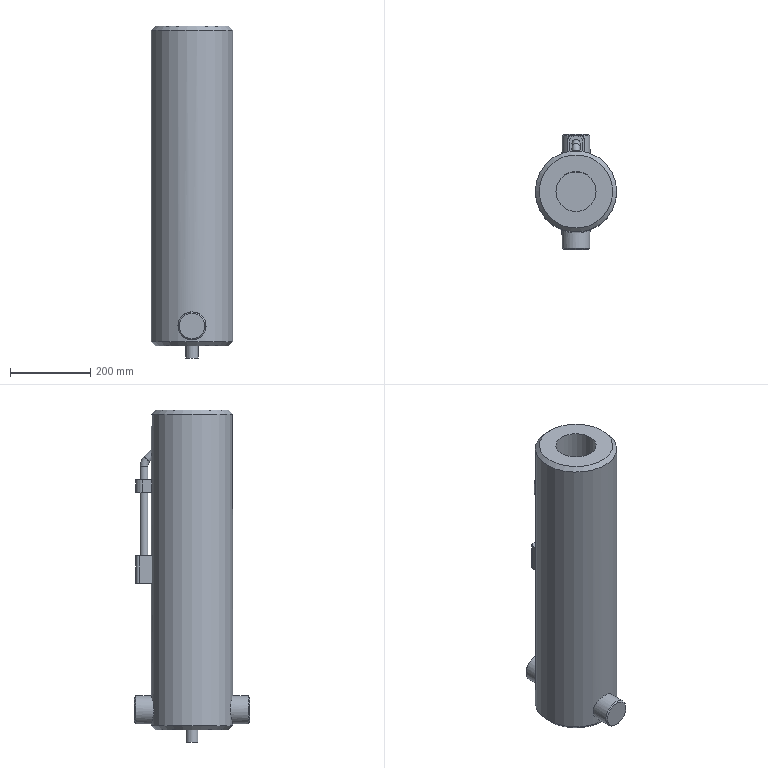Part | NX | features 护帮千斤顶缸 2 | 1 solid | 38 faces | box 203 x 287 x 828 mm | volume 20904449 mm3 | plane 17 | cylinder 14 | cone 6 | torus 1 | commonest cylinder face diameters 20 x3 10 x2 16 x2 34 x2 70 x2 30 x1
STEP:
#1=CARTESIAN_POINT('',(91.5,0.,0.));
#2=VERTEX_POINT('',#1);
#3=CARTESIAN_POINT('',(0.,0.,0.));
#4=DIRECTION('',(0.,0.,1.));
#5=DIRECTION('',(1.,0.,0.));
#6=AXIS2_PLACEMENT_3D('',#3,#4,#5);
#7=CIRCLE('',#6,91.5);
#8=EDGE_CURVE('',#2,#2,#7,.F.);
#9=ORIENTED_EDGE('',*,*,#8,.T.);
#10=EDGE_LOOP('',(#9));
#11=FACE_BOUND('',#10,.T.);
#12=CARTESIAN_POINT('',(15.,0.,0.));
#13=VERTEX_POINT('',#12);
#14=CARTESIAN_POINT('',(0.,0.,0.));
#15=DIRECTION('',(0.,0.,1.));
#16=DIRECTION('',(1.,0.,0.));
#17=AXIS2_PLACEMENT_3D('',#14,#15,#16);
#18=CIRCLE('',#17,15.);
#19=EDGE_CURVE('',#13,#13,#18,.F.);
#20=ORIENTED_EDGE('',*,*,#19,.F.);
#21=EDGE_LOOP('',(#20));
#22=FACE_BOUND('',#21,.T.);
#23=CARTESIAN_POINT('',(0.,0.,0.));
#24=DIRECTION('',(0.,0.,1.));
#25=DIRECTION('',(1.,0.,0.));
#26=AXIS2_PLACEMENT_3D('',#23,#24,#25);
#27=PLANE('',#26);
#28=ADVANCED_FACE('',(#11,#22),#27,.F.);
#29=CARTESIAN_POINT('',(20.,132.,434.5));
#30=VERTEX_POINT('',#29);
#31=CARTESIAN_POINT('',(20.,99.51,434.5));
#32=VERTEX_POINT('',#31);
#33=CARTESIAN_POINT('',(20.,140.,434.5));
#34=DIRECTION('',(0.,-1.,0.));
#35=VECTOR('',#34,1000.);
#36=LINE('',#33,#35);
#37=EDGE_CURVE('',#30,#32,#36,.T.);
#38=ORIENTED_EDGE('',*,*,#37,.F.);
#39=CARTESIAN_POINT('',(12.,140.,434.5));
#40=VERTEX_POINT('',#39);
#41=CARTESIAN_POINT('',(12.,132.,434.5));
#42=DIRECTION('',(0.,0.,-1.));
#43=DIRECTION('',(-1.,0.,0.));
#44=AXIS2_PLACEMENT_3D('',#41,#42,#43);
#45=CIRCLE('',#44,8.);
#46=EDGE_CURVE('',#30,#40,#45,.F.);
#47=ORIENTED_EDGE('',*,*,#46,.T.);
#48=CARTESIAN_POINT('',(-12.,140.,434.5));
#49=VERTEX_POINT('',#48);
#50=CARTESIAN_POINT('',(-20.,140.,434.5));
#51=DIRECTION('',(1.,0.,0.));
#52=VECTOR('',#51,1000.);
#53=LINE('',#50,#52);
#54=EDGE_CURVE('',#49,#40,#53,.T.);
#55=ORIENTED_EDGE('',*,*,#54,.F.);
#56=CARTESIAN_POINT('',(-20.,132.,434.5));
#57=VERTEX_POINT('',#56);
#58=CARTESIAN_POINT('',(-12.,132.,434.5));
#59=DIRECTION('',(0.,0.,-1.));
#60=DIRECTION('',(-1.,0.,0.));
#61=AXIS2_PLACEMENT_3D('',#58,#59,#60);
#62=CIRCLE('',#61,8.);
#63=EDGE_CURVE('',#49,#57,#62,.F.);
#64=ORIENTED_EDGE('',*,*,#63,.T.);
#65=CARTESIAN_POINT('',(-20.,99.51,434.5));
#66=VERTEX_POINT('',#65);
#67=CARTESIAN_POINT('',(-20.,140.,434.5));
#68=DIRECTION('',(0.,-1.,0.));
#69=VECTOR('',#68,1000.);
#70=LINE('',#67,#69);
#71=EDGE_CURVE('',#57,#66,#70,.T.);
#72=ORIENTED_EDGE('',*,*,#71,.T.);
#73=CARTESIAN_POINT('',(0.,0.,434.5));
#74=DIRECTION('',(0.,0.,-1.));
#75=DIRECTION('',(-1.,0.,0.));
#76=AXIS2_PLACEMENT_3D('',#73,#74,#75);
#77=CIRCLE('',#76,101.5);
#78=EDGE_CURVE('',#66,#32,#77,.T.);
#79=ORIENTED_EDGE('',*,*,#78,.T.);
#80=EDGE_LOOP('',(#38,#47,#55,#64,#72,#79));
#81=FACE_BOUND('',#80,.T.);
#82=CARTESIAN_POINT('',(10.,119.755,434.5));
#83=VERTEX_POINT('',#82);
#84=CARTESIAN_POINT('',(0.,119.755,434.5));
#85=DIRECTION('',(0.,0.,1.));
#86=DIRECTION('',(1.,0.,0.));
#87=AXIS2_PLACEMENT_3D('',#84,#85,#86);
#88=CIRCLE('',#87,10.);
#89=EDGE_CURVE('',#83,#83,#88,.T.);
#90=ORIENTED_EDGE('',*,*,#89,.F.);
#91=EDGE_LOOP('',(#90));
#92=FACE_BOUND('',#91,.T.);
#93=CARTESIAN_POINT('',(-20.,140.,434.5));
#94=DIRECTION('',(0.,0.,-1.));
#95=DIRECTION('',(-1.,0.,0.));
#96=AXIS2_PLACEMENT_3D('',#93,#94,#95);
#97=PLANE('',#96);
#98=ADVANCED_FACE('',(#81,#92),#97,.F.);
#99=CARTESIAN_POINT('',(17.,123.,624.17));
#100=VERTEX_POINT('',#99);
#101=CARTESIAN_POINT('',(17.,100.066,624.17));
#102=VERTEX_POINT('',#101);
#103=CARTESIAN_POINT('',(17.,140.,624.17));
#104=DIRECTION('',(0.,-1.,0.));
#105=VECTOR('',#104,1000.);
#106=LINE('',#103,#105);
#107=EDGE_CURVE('',#100,#102,#106,.T.);
#108=ORIENTED_EDGE('',*,*,#107,.F.);
#109=CARTESIAN_POINT('',(0.,140.,624.17));
#110=VERTEX_POINT('',#109);
#111=CARTESIAN_POINT('',(0.,123.,624.17));
#112=DIRECTION('',(0.,0.,-1.));
#113=DIRECTION('',(-1.,0.,0.));
#114=AXIS2_PLACEMENT_3D('',#111,#112,#113);
#115=CIRCLE('',#114,17.);
#116=EDGE_CURVE('',#100,#110,#115,.F.);
#117=ORIENTED_EDGE('',*,*,#116,.T.);
#118=CARTESIAN_POINT('',(-17.,123.,624.17));
#119=VERTEX_POINT('',#118);
#120=CARTESIAN_POINT('',(0.,123.,624.17));
#121=DIRECTION('',(0.,0.,-1.));
#122=DIRECTION('',(-1.,0.,0.));
#123=AXIS2_PLACEMENT_3D('',#120,#121,#122);
#124=CIRCLE('',#123,17.);
#125=EDGE_CURVE('',#110,#119,#124,.F.);
#126=ORIENTED_EDGE('',*,*,#125,.T.);
#127=CARTESIAN_POINT('',(-17.,100.066,624.17));
#128=VERTEX_POINT('',#127);
#129=CARTESIAN_POINT('',(-17.,140.,624.17));
#130=DIRECTION('',(0.,-1.,0.));
#131=VECTOR('',#130,1000.);
#132=LINE('',#129,#131);
#133=EDGE_CURVE('',#119,#128,#132,.T.);
#134=ORIENTED_EDGE('',*,*,#133,.T.);
#135=CARTESIAN_POINT('',(0.,0.,624.17));
#136=DIRECTION('',(0.,0.,-1.));
#137=DIRECTION('',(-1.,0.,0.));
#138=AXIS2_PLACEMENT_3D('',#135,#136,#137);
#139=CIRCLE('',#138,101.5);
#140=EDGE_CURVE('',#128,#102,#139,.T.);
#141=ORIENTED_EDGE('',*,*,#140,.T.);
#142=EDGE_LOOP('',(#108,#117,#126,#134,#141));
#143=FACE_BOUND('',#142,.T.);
#144=CARTESIAN_POINT('',(-10.,119.755,624.17));
#145=VERTEX_POINT('',#144);
#146=CARTESIAN_POINT('',(0.,119.755,624.17));
#147=DIRECTION('',(0.,0.,-1.));
#148=DIRECTION('',(-1.,0.,0.));
#149=AXIS2_PLACEMENT_3D('',#146,#147,#148);
#150=CIRCLE('',#149,10.);
#151=EDGE_CURVE('',#145,#145,#150,.F.);
#152=ORIENTED_EDGE('',*,*,#151,.F.);
#153=EDGE_LOOP('',(#152));
#154=FACE_BOUND('',#153,.T.);
#155=CARTESIAN_POINT('',(-17.,140.,624.17));
#156=DIRECTION('',(0.,0.,-1.));
#157=DIRECTION('',(-1.,0.,0.));
#158=AXIS2_PLACEMENT_3D('',#155,#156,#157);
#159=PLANE('',#158);
#160=ADVANCED_FACE('',(#143,#154),#159,.F.);
#161=CARTESIAN_POINT('',(-17.,123.,591.84));
#162=VERTEX_POINT('',#161);
#163=CARTESIAN_POINT('',(0.,140.,591.84));
#164=VERTEX_POINT('',#163);
#165=CARTESIAN_POINT('',(0.,123.,591.84));
#166=DIRECTION('',(0.,0.,1.));
#167=DIRECTION('',(1.,0.,0.));
#168=AXIS2_PLACEMENT_3D('',#165,#166,#167);
#169=CIRCLE('',#168,17.);
#170=EDGE_CURVE('',#162,#164,#169,.F.);
#171=ORIENTED_EDGE('',*,*,#170,.T.);
#172=CARTESIAN_POINT('',(17.,123.,591.84));
#173=VERTEX_POINT('',#172);
#174=CARTESIAN_POINT('',(0.,123.,591.84));
#175=DIRECTION('',(0.,0.,1.));
#176=DIRECTION('',(1.,0.,0.));
#177=AXIS2_PLACEMENT_3D('',#174,#175,#176);
#178=CIRCLE('',#177,17.);
#179=EDGE_CURVE('',#164,#173,#178,.F.);
#180=ORIENTED_EDGE('',*,*,#179,.T.);
#181=CARTESIAN_POINT('',(17.,100.066,591.84));
#182=VERTEX_POINT('',#181);
#183=CARTESIAN_POINT('',(17.,140.,591.84));
#184=DIRECTION('',(0.,-1.,0.));
#185=VECTOR('',#184,1000.);
#186=LINE('',#183,#185);
#187=EDGE_CURVE('',#173,#182,#186,.T.);
#188=ORIENTED_EDGE('',*,*,#187,.T.);
#189=CARTESIAN_POINT('',(-17.,100.066,591.84));
#190=VERTEX_POINT('',#189);
#191=CARTESIAN_POINT('',(0.,0.,591.84));
#192=DIRECTION('',(0.,0.,1.));
#193=DIRECTION('',(1.,0.,0.));
#194=AXIS2_PLACEMENT_3D('',#191,#192,#193);
#195=CIRCLE('',#194,101.5);
#196=EDGE_CURVE('',#182,#190,#195,.T.);
#197=ORIENTED_EDGE('',*,*,#196,.T.);
#198=CARTESIAN_POINT('',(-17.,140.,591.84));
#199=DIRECTION('',(0.,-1.,0.));
#200=VECTOR('',#199,1000.);
#201=LINE('',#198,#200);
#202=EDGE_CURVE('',#162,#190,#201,.T.);
#203=ORIENTED_EDGE('',*,*,#202,.F.);
#204=EDGE_LOOP('',(#171,#180,#188,#197,#203));
#205=FACE_BOUND('',#204,.T.);
#206=CARTESIAN_POINT('',(10.,119.755,591.84));
#207=VERTEX_POINT('',#206);
#208=CARTESIAN_POINT('',(0.,119.755,591.84));
#209=DIRECTION('',(0.,0.,1.));
#210=DIRECTION('',(1.,0.,0.));
#211=AXIS2_PLACEMENT_3D('',#208,#209,#210);
#212=CIRCLE('',#211,10.);
#213=EDGE_CURVE('',#207,#207,#212,.F.);
#214=ORIENTED_EDGE('',*,*,#213,.F.);
#215=EDGE_LOOP('',(#214));
#216=FACE_BOUND('',#215,.T.);
#217=CARTESIAN_POINT('',(-17.,140.,591.84));
#218=DIRECTION('',(0.,0.,1.));
#219=DIRECTION('',(1.,0.,0.));
#220=AXIS2_PLACEMENT_3D('',#217,#218,#219);
#221=PLANE('',#220);
#222=ADVANCED_FACE('',(#205,#216),#221,.F.);
#223=CARTESIAN_POINT('',(101.5,0.,788.));
#224=VERTEX_POINT('',#223);
#225=CARTESIAN_POINT('',(0.,0.,788.));
#226=DIRECTION('',(0.,0.,1.));
#227=DIRECTION('',(1.,0.,0.));
#228=AXIS2_PLACEMENT_3D('',#225,#226,#227);
#229=CIRCLE('',#228,101.5);
#230=EDGE_CURVE('',#224,#224,#229,.F.);
#231=ORIENTED_EDGE('',*,*,#230,.T.);
#232=EDGE_LOOP('',(#231));
#233=FACE_BOUND('',#232,.T.);
#234=CARTESIAN_POINT('',(0.,101.5,671.943));
#235=VERTEX_POINT('',#234);
#236=CARTESIAN_POINT('',(-2.408,101.48,672.245));
#237=CARTESIAN_POINT('',(0.8153,101.52,671.637));
#238=CARTESIAN_POINT('',(4.704,101.417,673.183));
#239=CARTESIAN_POINT('',(7.766,101.211,676.987));
#240=CARTESIAN_POINT('',(9.529,101.054,681.426));
#241=CARTESIAN_POINT('',(10.182,100.988,686.186));
#242=CARTESIAN_POINT('',(9.719,101.035,690.945));
#243=CARTESIAN_POINT('',(8.008,101.192,695.439));
#244=CARTESIAN_POINT('',(4.799,101.414,699.129));
#245=CARTESIAN_POINT('',(0.04319,101.542,700.764));
#246=CARTESIAN_POINT('',(-4.734,101.417,699.177));
#247=CARTESIAN_POINT('',(-7.971,101.195,695.504));
#248=CARTESIAN_POINT('',(-9.706,101.036,691.009));
#249=CARTESIAN_POINT('',(-10.185,100.987,686.22));
#250=CARTESIAN_POINT('',(-9.534,101.053,681.451));
#251=CARTESIAN_POINT('',(-7.788,101.21,677.014));
#252=CARTESIAN_POINT('',(-5.218,101.381,673.84));
#253=CARTESIAN_POINT('',(-2.408,101.48,672.245));
#254=CARTESIAN_POINT('',(0.8153,101.52,671.637));
#255=CARTESIAN_POINT('',(4.704,101.417,673.183));
#256=B_SPLINE_CURVE_WITH_KNOTS('',3,(#236,#237,#238,#239,#240,#241,#242,#243,#244,#245,#246,#247,#248,#249,#250,#251,#252,#253,#254,#255),.UNSPECIFIED.,.T.,.F.,(1,1,1,1,1,1,1,1,1,1,1,1,1,1,1,1,1,1,1,1,1,1,1,1),(-0.009513,-0.004756,-0.002378,0.,0.004756,0.009513,0.01427,0.01903,0.02378,0.02854,0.03329,0.03805,0.04281,0.04756,0.05232,0.05708,0.06183,0.06659,0.07134,0.07372,0.0761,0.08086,0.08561,0.09037),.UNSPECIFIED.);
#257=EDGE_CURVE('',#235,#235,#256,.T.);
#258=ORIENTED_EDGE('',*,*,#257,.T.);
#259=EDGE_LOOP('',(#258));
#260=FACE_BOUND('',#259,.T.);
#261=CARTESIAN_POINT('',(-20.,99.51,365.5));
#262=VERTEX_POINT('',#261);
#263=CARTESIAN_POINT('',(-20.,99.51,798.));
#264=DIRECTION('',(0.,0.,-1.));
#265=VECTOR('',#264,1000.);
#266=LINE('',#263,#265);
#267=EDGE_CURVE('',#262,#66,#266,.F.);
#268=ORIENTED_EDGE('',*,*,#267,.F.);
#269=CARTESIAN_POINT('',(20.,99.51,365.5));
#270=VERTEX_POINT('',#269);
#271=CARTESIAN_POINT('',(0.,0.,365.5));
#272=DIRECTION('',(0.,0.,1.));
#273=DIRECTION('',(1.,0.,0.));
#274=AXIS2_PLACEMENT_3D('',#271,#272,#273);
#275=CIRCLE('',#274,101.5);
#276=EDGE_CURVE('',#270,#262,#275,.T.);
#277=ORIENTED_EDGE('',*,*,#276,.F.);
#278=CARTESIAN_POINT('',(20.,99.51,798.));
#279=DIRECTION('',(0.,0.,-1.));
#280=VECTOR('',#279,1000.);
#281=LINE('',#278,#280);
#282=EDGE_CURVE('',#32,#270,#281,.T.);
#283=ORIENTED_EDGE('',*,*,#282,.F.);
#284=ORIENTED_EDGE('',*,*,#78,.F.);
#285=EDGE_LOOP('',(#268,#277,#283,#284));
#286=FACE_BOUND('',#285,.T.);
#287=CARTESIAN_POINT('',(101.5,0.,10.));
#288=VERTEX_POINT('',#287);
#289=CARTESIAN_POINT('',(0.,0.,10.));
#290=DIRECTION('',(0.,0.,1.));
#291=DIRECTION('',(1.,0.,0.));
#292=AXIS2_PLACEMENT_3D('',#289,#290,#291);
#293=CIRCLE('',#292,101.5);
#294=EDGE_CURVE('',#288,#288,#293,.T.);
#295=ORIENTED_EDGE('',*,*,#294,.T.);
#296=EDGE_LOOP('',(#295));
#297=FACE_BOUND('',#296,.T.);
#298=CARTESIAN_POINT('',(0.,-101.5,15.));
#299=VERTEX_POINT('',#298);
#300=CARTESIAN_POINT('',(-13.849,-100.835,16.867));
#301=CARTESIAN_POINT('',(-0.001134,-101.833,14.067));
#302=CARTESIAN_POINT('',(13.853,-100.834,16.867));
#303=CARTESIAN_POINT('',(25.391,-98.445,24.635));
#304=CARTESIAN_POINT('',(33.131,-95.991,36.158));
#305=CARTESIAN_POINT('',(35.93,-94.918,49.967));
#306=CARTESIAN_POINT('',(33.147,-95.985,63.826));
#307=CARTESIAN_POINT('',(25.374,-98.45,75.386));
#308=CARTESIAN_POINT('',(13.835,-100.836,83.136));
#309=CARTESIAN_POINT('',(0.01694,-101.831,85.93));
#310=CARTESIAN_POINT('',(-13.822,-100.839,83.145));
#311=CARTESIAN_POINT('',(-25.383,-98.447,75.386));
#312=CARTESIAN_POINT('',(-31.849,-96.4,65.731));
#313=CARTESIAN_POINT('',(-34.534,-95.448,56.956));
#314=CARTESIAN_POINT('',(-35.466,-95.099,47.672));
#315=CARTESIAN_POINT('',(-33.138,-95.987,36.172));
#316=CARTESIAN_POINT('',(-25.383,-98.448,24.623));
#317=CARTESIAN_POINT('',(-13.849,-100.835,16.867));
#318=CARTESIAN_POINT('',(-0.001134,-101.833,14.067));
#319=CARTESIAN_POINT('',(13.853,-100.834,16.867));
#320=B_SPLINE_CURVE_WITH_KNOTS('',3,(#300,#301,#302,#303,#304,#305,#306,#307,#308,#309,#310,#311,#312,#313,#314,#315,#316,#317,#318,#319),.UNSPECIFIED.,.T.,.F.,(1,1,1,1,1,1,1,1,1,1,1,1,1,1,1,1,1,1,1,1,1,1,1,1),(-0.04135,-0.02757,-0.01378,0.,0.01378,0.02757,0.04135,0.05513,0.06892,0.0827,0.09648,0.1103,0.124,0.1378,0.1516,0.1585,0.1654,0.1792,0.193,0.2067,0.2205,0.2343,0.2481,0.2619),.UNSPECIFIED.);
#321=EDGE_CURVE('',#299,#299,#320,.T.);
#322=ORIENTED_EDGE('',*,*,#321,.F.);
#323=EDGE_LOOP('',(#322));
#324=FACE_BOUND('',#323,.T.);
#325=CARTESIAN_POINT('',(0.,101.5,15.));
#326=VERTEX_POINT('',#325);
#327=CARTESIAN_POINT('',(13.849,100.835,16.867));
#328=CARTESIAN_POINT('',(0.001134,101.833,14.067));
#329=CARTESIAN_POINT('',(-13.853,100.834,16.867));
#330=CARTESIAN_POINT('',(-25.391,98.445,24.635));
#331=CARTESIAN_POINT('',(-33.131,95.991,36.158));
#332=CARTESIAN_POINT('',(-35.93,94.918,49.967));
#333=CARTESIAN_POINT('',(-33.147,95.985,63.826));
#334=CARTESIAN_POINT('',(-25.374,98.45,75.386));
#335=CARTESIAN_POINT('',(-13.835,100.836,83.136));
#336=CARTESIAN_POINT('',(-0.01694,101.831,85.93));
#337=CARTESIAN_POINT('',(13.822,100.839,83.145));
#338=CARTESIAN_POINT('',(25.383,98.447,75.386));
#339=CARTESIAN_POINT('',(31.849,96.4,65.731));
#340=CARTESIAN_POINT('',(34.534,95.448,56.956));
#341=CARTESIAN_POINT('',(35.466,95.099,47.672));
#342=CARTESIAN_POINT('',(33.138,95.987,36.172));
#343=CARTESIAN_POINT('',(25.383,98.448,24.623));
#344=CARTESIAN_POINT('',(13.849,100.835,16.867));
#345=CARTESIAN_POINT('',(0.001134,101.833,14.067));
#346=CARTESIAN_POINT('',(-13.853,100.834,16.867));
#347=B_SPLINE_CURVE_WITH_KNOTS('',3,(#327,#328,#329,#330,#331,#332,#333,#334,#335,#336,#337,#338,#339,#340,#341,#342,#343,#344,#345,#346),.UNSPECIFIED.,.T.,.F.,(1,1,1,1,1,1,1,1,1,1,1,1,1,1,1,1,1,1,1,1,1,1,1,1),(-0.04135,-0.02757,-0.01378,0.,0.01378,0.02757,0.04135,0.05513,0.06892,0.0827,0.09648,0.1103,0.124,0.1378,0.1516,0.1585,0.1654,0.1792,0.193,0.2067,0.2205,0.2343,0.2481,0.2619),.UNSPECIFIED.);
#348=EDGE_CURVE('',#326,#326,#347,.T.);
#349=ORIENTED_EDGE('',*,*,#348,.F.);
#350=EDGE_LOOP('',(#349));
#351=FACE_BOUND('',#350,.T.);
#352=CARTESIAN_POINT('',(-17.,100.066,798.));
#353=DIRECTION('',(0.,0.,-1.));
#354=VECTOR('',#353,1000.);
#355=LINE('',#352,#354);
#356=EDGE_CURVE('',#190,#128,#355,.F.);
#357=ORIENTED_EDGE('',*,*,#356,.F.);
#358=ORIENTED_EDGE('',*,*,#196,.F.);
#359=CARTESIAN_POINT('',(17.,100.066,798.));
#360=DIRECTION('',(0.,0.,-1.));
#361=VECTOR('',#360,1000.);
#362=LINE('',#359,#361);
#363=EDGE_CURVE('',#102,#182,#362,.T.);
#364=ORIENTED_EDGE('',*,*,#363,.F.);
#365=ORIENTED_EDGE('',*,*,#140,.F.);
#366=EDGE_LOOP('',(#357,#358,#364,#365));
#367=FACE_BOUND('',#366,.T.);
#368=CARTESIAN_POINT('',(0.,0.,798.));
#369=DIRECTION('',(0.,0.,-1.));
#370=DIRECTION('',(-1.,0.,0.));
#371=AXIS2_PLACEMENT_3D('',#368,#369,#370);
#372=CYLINDRICAL_SURFACE('',#371,101.5);
#373=ADVANCED_FACE('',(#233,#260,#286,#297,#324,#351,#367),#372,.T.);
#374=CARTESIAN_POINT('',(91.5,0.,798.));
#375=VERTEX_POINT('',#374);
#376=CARTESIAN_POINT('',(0.,0.,798.));
#377=DIRECTION('',(0.,0.,1.));
#378=DIRECTION('',(1.,0.,0.));
#379=AXIS2_PLACEMENT_3D('',#376,#377,#378);
#380=CIRCLE('',#379,91.5);
#381=EDGE_CURVE('',#375,#375,#380,.T.);
#382=ORIENTED_EDGE('',*,*,#381,.T.);
#383=EDGE_LOOP('',(#382));
#384=FACE_BOUND('',#383,.T.);
#385=CARTESIAN_POINT('',(50.,0.,798.));
#386=VERTEX_POINT('',#385);
#387=CARTESIAN_POINT('',(0.,0.,798.));
#388=DIRECTION('',(0.,0.,1.));
#389=DIRECTION('',(1.,0.,0.));
#390=AXIS2_PLACEMENT_3D('',#387,#388,#389);
#391=CIRCLE('',#390,50.);
#392=EDGE_CURVE('',#386,#386,#391,.T.);
#393=ORIENTED_EDGE('',*,*,#392,.F.);
#394=EDGE_LOOP('',(#393));
#395=FACE_BOUND('',#394,.T.);
#396=CARTESIAN_POINT('',(0.,0.,798.));
#397=DIRECTION('',(0.,0.,1.));
#398=DIRECTION('',(1.,0.,0.));
#399=AXIS2_PLACEMENT_3D('',#396,#397,#398);
#400=PLANE('',#399);
#401=ADVANCED_FACE('',(#384,#395),#400,.T.);
#402=CARTESIAN_POINT('',(0.,-143.5,82.));
#403=VERTEX_POINT('',#402);
#404=CARTESIAN_POINT('',(0.,-143.5,50.));
#405=DIRECTION('',(0.,1.,0.));
#406=DIRECTION('',(0.,0.,1.));
#407=AXIS2_PLACEMENT_3D('',#404,#405,#406);
#408=CIRCLE('',#407,32.);
#409=EDGE_CURVE('',#403,#403,#408,.F.);
#410=ORIENTED_EDGE('',*,*,#409,.T.);
#411=EDGE_LOOP('',(#410));
#412=FACE_BOUND('',#411,.T.);
#413=CARTESIAN_POINT('',(0.,-143.5,50.));
#414=DIRECTION('',(0.,1.,0.));
#415=DIRECTION('',(0.,0.,1.));
#416=AXIS2_PLACEMENT_3D('',#413,#414,#415);
#417=PLANE('',#416);
#418=ADVANCED_FACE('',(#412),#417,.F.);
#419=CARTESIAN_POINT('',(0.,-140.5,85.));
#420=VERTEX_POINT('',#419);
#421=CARTESIAN_POINT('',(0.,-140.5,50.));
#422=DIRECTION('',(0.,1.,0.));
#423=DIRECTION('',(0.,0.,1.));
#424=AXIS2_PLACEMENT_3D('',#421,#422,#423);
#425=CIRCLE('',#424,35.);
#426=EDGE_CURVE('',#420,#420,#425,.T.);
#427=ORIENTED_EDGE('',*,*,#426,.T.);
#428=EDGE_LOOP('',(#427));
#429=FACE_BOUND('',#428,.T.);
#430=ORIENTED_EDGE('',*,*,#321,.T.);
#431=EDGE_LOOP('',(#430));
#432=FACE_BOUND('',#431,.T.);
#433=CARTESIAN_POINT('',(0.,143.5,50.));
#434=DIRECTION('',(0.,-1.,0.));
#435=DIRECTION('',(0.,0.,-1.));
#436=AXIS2_PLACEMENT_3D('',#433,#434,#435);
#437=CYLINDRICAL_SURFACE('',#436,35.);
#438=ADVANCED_FACE('',(#429,#432),#437,.T.);
#439=CARTESIAN_POINT('',(0.,140.5,85.));
#440=VERTEX_POINT('',#439);
#441=CARTESIAN_POINT('',(0.,140.5,50.));
#442=DIRECTION('',(0.,1.,0.));
#443=DIRECTION('',(0.,0.,1.));
#444=AXIS2_PLACEMENT_3D('',#441,#442,#443);
#445=CIRCLE('',#444,35.);
#446=EDGE_CURVE('',#440,#440,#445,.F.);
#447=ORIENTED_EDGE('',*,*,#446,.T.);
#448=EDGE_LOOP('',(#447));
#449=FACE_BOUND('',#448,.T.);
#450=ORIENTED_EDGE('',*,*,#348,.T.);
#451=EDGE_LOOP('',(#450));
#452=FACE_BOUND('',#451,.T.);
#453=CARTESIAN_POINT('',(0.,143.5,50.));
#454=DIRECTION('',(0.,-1.,0.));
#455=DIRECTION('',(0.,0.,-1.));
#456=AXIS2_PLACEMENT_3D('',#453,#454,#455);
#457=CYLINDRICAL_SURFACE('',#456,35.);
#458=ADVANCED_FACE('',(#449,#452),#457,.T.);
#459=CARTESIAN_POINT('',(0.,143.5,82.));
#460=VERTEX_POINT('',#459);
#461=CARTESIAN_POINT('',(0.,143.5,50.));
#462=DIRECTION('',(0.,1.,0.));
#463=DIRECTION('',(0.,0.,1.));
#464=AXIS2_PLACEMENT_3D('',#461,#462,#463);
#465=CIRCLE('',#464,32.);
#466=EDGE_CURVE('',#460,#460,#465,.T.);
#467=ORIENTED_EDGE('',*,*,#466,.T.);
#468=EDGE_LOOP('',(#467));
#469=FACE_BOUND('',#468,.T.);
#470=CARTESIAN_POINT('',(0.,143.5,50.));
#471=DIRECTION('',(0.,1.,0.));
#472=DIRECTION('',(0.,0.,1.));
#473=AXIS2_PLACEMENT_3D('',#470,#471,#472);
#474=PLANE('',#473);
#475=ADVANCED_FACE('',(#469),#474,.T.);
#476=ORIENTED_EDGE('',*,*,#409,.F.);
#477=EDGE_LOOP('',(#476));
#478=FACE_BOUND('',#477,.T.);
#479=ORIENTED_EDGE('',*,*,#426,.F.);
#480=EDGE_LOOP('',(#479));
#481=FACE_BOUND('',#480,.T.);
#482=CARTESIAN_POINT('',(0.,-140.5,50.));
#483=DIRECTION('',(0.,1.,0.));
#484=DIRECTION('',(0.,0.,1.));
#485=AXIS2_PLACEMENT_3D('',#482,#483,#484);
#486=CONICAL_SURFACE('',#485,35.,0.7854);
#487=ADVANCED_FACE('',(#478,#481),#486,.T.);
#488=ORIENTED_EDGE('',*,*,#446,.F.);
#489=EDGE_LOOP('',(#488));
#490=FACE_BOUND('',#489,.T.);
#491=ORIENTED_EDGE('',*,*,#466,.F.);
#492=EDGE_LOOP('',(#491));
#493=FACE_BOUND('',#492,.T.);
#494=CARTESIAN_POINT('',(0.,143.5,50.));
#495=DIRECTION('',(0.,-1.,0.));
#496=DIRECTION('',(0.,0.,-1.));
#497=AXIS2_PLACEMENT_3D('',#494,#495,#496);
#498=CONICAL_SURFACE('',#497,32.,0.7854);
#499=ADVANCED_FACE('',(#490,#493),#498,.T.);
#500=ORIENTED_EDGE('',*,*,#8,.F.);
#501=EDGE_LOOP('',(#500));
#502=FACE_BOUND('',#501,.T.);
#503=ORIENTED_EDGE('',*,*,#294,.F.);
#504=EDGE_LOOP('',(#503));
#505=FACE_BOUND('',#504,.T.);
#506=CARTESIAN_POINT('',(0.,0.,10.));
#507=DIRECTION('',(0.,0.,1.));
#508=DIRECTION('',(1.,0.,0.));
#509=AXIS2_PLACEMENT_3D('',#506,#507,#508);
#510=CONICAL_SURFACE('',#509,101.5,0.7854);
#511=ADVANCED_FACE('',(#502,#505),#510,.T.);
#512=ORIENTED_EDGE('',*,*,#71,.F.);
#513=CARTESIAN_POINT('',(-20.,132.,365.5));
#514=VERTEX_POINT('',#513);
#515=CARTESIAN_POINT('',(-20.,132.,365.5));
#516=DIRECTION('',(0.,0.,1.));
#517=VECTOR('',#516,1000.);
#518=LINE('',#515,#517);
#519=EDGE_CURVE('',#57,#514,#518,.F.);
#520=ORIENTED_EDGE('',*,*,#519,.T.);
#521=CARTESIAN_POINT('',(-20.,140.,365.5));
#522=DIRECTION('',(0.,-1.,0.));
#523=VECTOR('',#522,1000.);
#524=LINE('',#521,#523);
#525=EDGE_CURVE('',#514,#262,#524,.T.);
#526=ORIENTED_EDGE('',*,*,#525,.T.);
#527=ORIENTED_EDGE('',*,*,#267,.T.);
#528=EDGE_LOOP('',(#512,#520,#526,#527));
#529=FACE_BOUND('',#528,.T.);
#530=CARTESIAN_POINT('',(-20.,140.,365.5));
#531=DIRECTION('',(1.,0.,0.));
#532=DIRECTION('',(0.,0.,-1.));
#533=AXIS2_PLACEMENT_3D('',#530,#531,#532);
#534=PLANE('',#533);
#535=ADVANCED_FACE('',(#529),#534,.F.);
#536=CARTESIAN_POINT('',(20.,132.,365.5));
#537=VERTEX_POINT('',#536);
#538=CARTESIAN_POINT('',(20.,140.,365.5));
#539=DIRECTION('',(0.,-1.,0.));
#540=VECTOR('',#539,1000.);
#541=LINE('',#538,#540);
#542=EDGE_CURVE('',#537,#270,#541,.T.);
#543=ORIENTED_EDGE('',*,*,#542,.F.);
#544=CARTESIAN_POINT('',(20.,132.,434.5));
#545=DIRECTION('',(0.,0.,-1.));
#546=VECTOR('',#545,1000.);
#547=LINE('',#544,#546);
#548=EDGE_CURVE('',#537,#30,#547,.F.);
#549=ORIENTED_EDGE('',*,*,#548,.T.);
#550=ORIENTED_EDGE('',*,*,#37,.T.);
#551=ORIENTED_EDGE('',*,*,#282,.T.);
#552=EDGE_LOOP('',(#543,#549,#550,#551));
#553=FACE_BOUND('',#552,.T.);
#554=CARTESIAN_POINT('',(20.,140.,365.5));
#555=DIRECTION('',(-1.,0.,0.));
#556=DIRECTION('',(0.,0.,1.));
#557=AXIS2_PLACEMENT_3D('',#554,#555,#556);
#558=PLANE('',#557);
#559=ADVANCED_FACE('',(#553),#558,.F.);
#560=CARTESIAN_POINT('',(12.,140.,365.5));
#561=VERTEX_POINT('',#560);
#562=CARTESIAN_POINT('',(-12.,140.,365.5));
#563=VERTEX_POINT('',#562);
#564=CARTESIAN_POINT('',(-20.,140.,365.5));
#565=DIRECTION('',(-1.,0.,0.));
#566=VECTOR('',#565,1000.);
#567=LINE('',#564,#566);
#568=EDGE_CURVE('',#561,#563,#567,.T.);
#569=ORIENTED_EDGE('',*,*,#568,.F.);
#570=CARTESIAN_POINT('',(12.,132.,365.5));
#571=DIRECTION('',(0.,0.,1.));
#572=DIRECTION('',(1.,0.,0.));
#573=AXIS2_PLACEMENT_3D('',#570,#571,#572);
#574=CIRCLE('',#573,8.);
#575=EDGE_CURVE('',#561,#537,#574,.F.);
#576=ORIENTED_EDGE('',*,*,#575,.T.);
#577=ORIENTED_EDGE('',*,*,#542,.T.);
#578=ORIENTED_EDGE('',*,*,#276,.T.);
#579=ORIENTED_EDGE('',*,*,#525,.F.);
#580=CARTESIAN_POINT('',(-12.,132.,365.5));
#581=DIRECTION('',(0.,0.,1.));
#582=DIRECTION('',(1.,0.,0.));
#583=AXIS2_PLACEMENT_3D('',#580,#581,#582);
#584=CIRCLE('',#583,8.);
#585=EDGE_CURVE('',#514,#563,#584,.F.);
#586=ORIENTED_EDGE('',*,*,#585,.T.);
#587=EDGE_LOOP('',(#569,#576,#577,#578,#579,#586));
#588=FACE_BOUND('',#587,.T.);
#589=CARTESIAN_POINT('',(-20.,140.,365.5));
#590=DIRECTION('',(0.,0.,1.));
#591=DIRECTION('',(1.,0.,0.));
#592=AXIS2_PLACEMENT_3D('',#589,#590,#591);
#593=PLANE('',#592);
#594=ADVANCED_FACE('',(#588),#593,.F.);
#595=CARTESIAN_POINT('',(0.,140.,427.17));
#596=VERTEX_POINT('',#595);
#597=CARTESIAN_POINT('',(0.,140.,421.17));
#598=DIRECTION('',(0.,1.,0.));
#599=DIRECTION('',(0.,0.,1.));
#600=AXIS2_PLACEMENT_3D('',#597,#598,#599);
#601=CIRCLE('',#600,6.);
#602=EDGE_CURVE('',#596,#596,#601,.F.);
#603=ORIENTED_EDGE('',*,*,#602,.T.);
#604=EDGE_LOOP('',(#603));
#605=FACE_BOUND('',#604,.T.);
#606=CARTESIAN_POINT('',(0.,140.,380.5));
#607=VERTEX_POINT('',#606);
#608=CARTESIAN_POINT('',(0.,140.,374.5));
#609=DIRECTION('',(0.,1.,0.));
#610=DIRECTION('',(0.,0.,1.));
#611=AXIS2_PLACEMENT_3D('',#608,#609,#610);
#612=CIRCLE('',#611,6.);
#613=EDGE_CURVE('',#607,#607,#612,.F.);
#614=ORIENTED_EDGE('',*,*,#613,.T.);
#615=EDGE_LOOP('',(#614));
#616=FACE_BOUND('',#615,.T.);
#617=ORIENTED_EDGE('',*,*,#54,.T.);
#618=CARTESIAN_POINT('',(12.,140.,365.5));
#619=DIRECTION('',(0.,0.,-1.));
#620=VECTOR('',#619,1000.);
#621=LINE('',#618,#620);
#622=EDGE_CURVE('',#40,#561,#621,.T.);
#623=ORIENTED_EDGE('',*,*,#622,.T.);
#624=ORIENTED_EDGE('',*,*,#568,.T.);
#625=CARTESIAN_POINT('',(-12.,140.,434.5));
#626=DIRECTION('',(0.,0.,1.));
#627=VECTOR('',#626,1000.);
#628=LINE('',#625,#627);
#629=EDGE_CURVE('',#563,#49,#628,.T.);
#630=ORIENTED_EDGE('',*,*,#629,.T.);
#631=EDGE_LOOP('',(#617,#623,#624,#630));
#632=FACE_BOUND('',#631,.T.);
#633=CARTESIAN_POINT('',(-20.,140.,434.5));
#634=DIRECTION('',(0.,1.,0.));
#635=DIRECTION('',(0.,0.,1.));
#636=AXIS2_PLACEMENT_3D('',#633,#634,#635);
#637=PLANE('',#636);
#638=ADVANCED_FACE('',(#605,#616,#632),#637,.T.);
#639=ORIENTED_EDGE('',*,*,#133,.F.);
#640=CARTESIAN_POINT('',(-17.,123.,591.84));
#641=DIRECTION('',(0.,0.,1.));
#642=VECTOR('',#641,1000.);
#643=LINE('',#640,#642);
#644=EDGE_CURVE('',#119,#162,#643,.F.);
#645=ORIENTED_EDGE('',*,*,#644,.T.);
#646=ORIENTED_EDGE('',*,*,#202,.T.);
#647=ORIENTED_EDGE('',*,*,#356,.T.);
#648=EDGE_LOOP('',(#639,#645,#646,#647));
#649=FACE_BOUND('',#648,.T.);
#650=CARTESIAN_POINT('',(-17.,140.,591.84));
#651=DIRECTION('',(1.,0.,0.));
#652=DIRECTION('',(0.,0.,-1.));
#653=AXIS2_PLACEMENT_3D('',#650,#651,#652);
#654=PLANE('',#653);
#655=ADVANCED_FACE('',(#649),#654,.F.);
#656=ORIENTED_EDGE('',*,*,#187,.F.);
#657=CARTESIAN_POINT('',(17.,123.,624.17));
#658=DIRECTION('',(0.,0.,-1.));
#659=VECTOR('',#658,1000.);
#660=LINE('',#657,#659);
#661=EDGE_CURVE('',#173,#100,#660,.F.);
#662=ORIENTED_EDGE('',*,*,#661,.T.);
#663=ORIENTED_EDGE('',*,*,#107,.T.);
#664=ORIENTED_EDGE('',*,*,#363,.T.);
#665=EDGE_LOOP('',(#656,#662,#663,#664));
#666=FACE_BOUND('',#665,.T.);
#667=CARTESIAN_POINT('',(17.,140.,591.84));
#668=DIRECTION('',(-1.,0.,0.));
#669=DIRECTION('',(0.,0.,1.));
#670=AXIS2_PLACEMENT_3D('',#667,#668,#669);
#671=PLANE('',#670);
#672=ADVANCED_FACE('',(#666),#671,.F.);
#673=ORIENTED_EDGE('',*,*,#89,.T.);
#674=EDGE_LOOP('',(#673));
#675=FACE_BOUND('',#674,.T.);
#676=ORIENTED_EDGE('',*,*,#213,.T.);
#677=EDGE_LOOP('',(#676));
#678=FACE_BOUND('',#677,.T.);
#679=CARTESIAN_POINT('',(0.,119.755,657.475));
#680=DIRECTION('',(0.,0.,-1.));
#681=DIRECTION('',(0.,1.,0.));
#682=AXIS2_PLACEMENT_3D('',#679,#680,#681);
#683=CYLINDRICAL_SURFACE('',#682,10.);
#684=ADVANCED_FACE('',(#675,#678),#683,.T.);
#685=CARTESIAN_POINT('',(10.,112.433,675.152));
#686=VERTEX_POINT('',#685);
#687=CARTESIAN_POINT('',(0.,112.433,675.152));
#688=DIRECTION('',(0.,-0.7071,0.7071));
#689=DIRECTION('',(1.,0.,0.));
#690=AXIS2_PLACEMENT_3D('',#687,#688,#689);
#691=CIRCLE('',#690,10.);
#692=EDGE_CURVE('',#686,#686,#691,.T.);
#693=ORIENTED_EDGE('',*,*,#692,.T.);
#694=EDGE_LOOP('',(#693));
#695=FACE_BOUND('',#694,.T.);
#696=ORIENTED_EDGE('',*,*,#257,.F.);
#697=EDGE_LOOP('',(#696));
#698=FACE_BOUND('',#697,.T.);
#699=CARTESIAN_POINT('',(0.,112.433,675.152));
#700=DIRECTION('',(0.,-0.7071,0.7071));
#701=DIRECTION('',(0.,-0.7071,-0.7071));
#702=AXIS2_PLACEMENT_3D('',#699,#700,#701);
#703=CYLINDRICAL_SURFACE('',#702,10.);
#704=ADVANCED_FACE('',(#695,#698),#703,.T.);
#705=CARTESIAN_POINT('',(10.,119.755,657.475));
#706=VERTEX_POINT('',#705);
#707=CARTESIAN_POINT('',(0.,119.755,657.475));
#708=DIRECTION('',(0.,0.,1.));
#709=DIRECTION('',(1.,0.,0.));
#710=AXIS2_PLACEMENT_3D('',#707,#708,#709);
#711=CIRCLE('',#710,10.);
#712=EDGE_CURVE('',#706,#706,#711,.T.);
#713=ORIENTED_EDGE('',*,*,#712,.F.);
#714=EDGE_LOOP('',(#713));
#715=FACE_BOUND('',#714,.T.);
#716=ORIENTED_EDGE('',*,*,#151,.T.);
#717=EDGE_LOOP('',(#716));
#718=FACE_BOUND('',#717,.T.);
#719=CARTESIAN_POINT('',(0.,119.755,657.475));
#720=DIRECTION('',(0.,0.,-1.));
#721=DIRECTION('',(0.,1.,0.));
#722=AXIS2_PLACEMENT_3D('',#719,#720,#721);
#723=CYLINDRICAL_SURFACE('',#722,10.);
#724=ADVANCED_FACE('',(#715,#718),#723,.T.);
#725=ORIENTED_EDGE('',*,*,#712,.T.);
#726=EDGE_LOOP('',(#725));
#727=FACE_BOUND('',#726,.T.);
#728=ORIENTED_EDGE('',*,*,#692,.F.);
#729=EDGE_LOOP('',(#728));
#730=FACE_BOUND('',#729,.T.);
#731=CARTESIAN_POINT('',(0.,94.755,657.475));
#732=DIRECTION('',(1.,0.,0.));
#733=DIRECTION('',(0.,0.,-1.));
#734=AXIS2_PLACEMENT_3D('',#731,#732,#733);
#735=TOROIDAL_SURFACE('',#734,25.,10.);
#736=ADVANCED_FACE('',(#727,#730),#735,.T.);
#737=ORIENTED_EDGE('',*,*,#644,.F.);
#738=ORIENTED_EDGE('',*,*,#125,.F.);
#739=CARTESIAN_POINT('',(0.,140.,624.17));
#740=DIRECTION('',(0.,0.,1.));
#741=VECTOR('',#740,1000.);
#742=LINE('',#739,#741);
#743=EDGE_CURVE('',#164,#110,#742,.T.);
#744=ORIENTED_EDGE('',*,*,#743,.F.);
#745=ORIENTED_EDGE('',*,*,#170,.F.);
#746=EDGE_LOOP('',(#737,#738,#744,#745));
#747=FACE_BOUND('',#746,.T.);
#748=CARTESIAN_POINT('',(0.,123.,624.17));
#749=DIRECTION('',(0.,0.,-1.));
#750=DIRECTION('',(-1.,0.,0.));
#751=AXIS2_PLACEMENT_3D('',#748,#749,#750);
#752=CYLINDRICAL_SURFACE('',#751,17.);
#753=ADVANCED_FACE('',(#747),#752,.T.);
#754=ORIENTED_EDGE('',*,*,#116,.F.);
#755=ORIENTED_EDGE('',*,*,#661,.F.);
#756=ORIENTED_EDGE('',*,*,#179,.F.);
#757=ORIENTED_EDGE('',*,*,#743,.T.);
#758=EDGE_LOOP('',(#754,#755,#756,#757));
#759=FACE_BOUND('',#758,.T.);
#760=CARTESIAN_POINT('',(0.,123.,624.17));
#761=DIRECTION('',(0.,0.,1.));
#762=DIRECTION('',(1.,0.,0.));
#763=AXIS2_PLACEMENT_3D('',#760,#761,#762);
#764=CYLINDRICAL_SURFACE('',#763,17.);
#765=ADVANCED_FACE('',(#759),#764,.T.);
#766=CARTESIAN_POINT('',(0.,139.,379.5));
#767=VERTEX_POINT('',#766);
#768=CARTESIAN_POINT('',(0.,139.,374.5));
#769=DIRECTION('',(0.,1.,0.));
#770=DIRECTION('',(0.,0.,1.));
#771=AXIS2_PLACEMENT_3D('',#768,#769,#770);
#772=CIRCLE('',#771,5.);
#773=EDGE_CURVE('',#767,#767,#772,.T.);
#774=ORIENTED_EDGE('',*,*,#773,.T.);
#775=EDGE_LOOP('',(#774));
#776=FACE_BOUND('',#775,.T.);
#777=CARTESIAN_POINT('',(0.,110.,379.5));
#778=VERTEX_POINT('',#777);
#779=CARTESIAN_POINT('',(0.,110.,374.5));
#780=DIRECTION('',(0.,1.,0.));
#781=DIRECTION('',(0.,0.,1.));
#782=AXIS2_PLACEMENT_3D('',#779,#780,#781);
#783=CIRCLE('',#782,5.);
#784=EDGE_CURVE('',#778,#778,#783,.T.);
#785=ORIENTED_EDGE('',*,*,#784,.F.);
#786=EDGE_LOOP('',(#785));
#787=FACE_BOUND('',#786,.T.);
#788=CARTESIAN_POINT('',(0.,110.,374.5));
#789=DIRECTION('',(0.,1.,0.));
#790=DIRECTION('',(0.,0.,1.));
#791=AXIS2_PLACEMENT_3D('',#788,#789,#790);
#792=CYLINDRICAL_SURFACE('',#791,5.);
#793=ADVANCED_FACE('',(#776,#787),#792,.F.);
#794=ORIENTED_EDGE('',*,*,#784,.T.);
#795=EDGE_LOOP('',(#794));
#796=FACE_BOUND('',#795,.T.);
#797=CARTESIAN_POINT('',(0.,110.,374.5));
#798=DIRECTION('',(0.,1.,0.));
#799=DIRECTION('',(0.,0.,1.));
#800=AXIS2_PLACEMENT_3D('',#797,#798,#799);
#801=PLANE('',#800);
#802=ADVANCED_FACE('',(#796),#801,.T.);
#803=CARTESIAN_POINT('',(0.,139.,426.17));
#804=VERTEX_POINT('',#803);
#805=CARTESIAN_POINT('',(0.,139.,421.17));
#806=DIRECTION('',(0.,1.,0.));
#807=DIRECTION('',(0.,0.,1.));
#808=AXIS2_PLACEMENT_3D('',#805,#806,#807);
#809=CIRCLE('',#808,5.);
#810=EDGE_CURVE('',#804,#804,#809,.T.);
#811=ORIENTED_EDGE('',*,*,#810,.T.);
#812=EDGE_LOOP('',(#811));
#813=FACE_BOUND('',#812,.T.);
#814=CARTESIAN_POINT('',(0.,110.,426.17));
#815=VERTEX_POINT('',#814);
#816=CARTESIAN_POINT('',(0.,110.,421.17));
#817=DIRECTION('',(0.,1.,0.));
#818=DIRECTION('',(0.,0.,1.));
#819=AXIS2_PLACEMENT_3D('',#816,#817,#818);
#820=CIRCLE('',#819,5.);
#821=EDGE_CURVE('',#815,#815,#820,.T.);
#822=ORIENTED_EDGE('',*,*,#821,.F.);
#823=EDGE_LOOP('',(#822));
#824=FACE_BOUND('',#823,.T.);
#825=CARTESIAN_POINT('',(0.,110.,421.17));
#826=DIRECTION('',(0.,1.,0.));
#827=DIRECTION('',(0.,0.,1.));
#828=AXIS2_PLACEMENT_3D('',#825,#826,#827);
#829=CYLINDRICAL_SURFACE('',#828,5.);
#830=ADVANCED_FACE('',(#813,#824),#829,.F.);
#831=ORIENTED_EDGE('',*,*,#821,.T.);
#832=EDGE_LOOP('',(#831));
#833=FACE_BOUND('',#832,.T.);
#834=CARTESIAN_POINT('',(0.,110.,421.17));
#835=DIRECTION('',(0.,1.,0.));
#836=DIRECTION('',(0.,0.,1.));
#837=AXIS2_PLACEMENT_3D('',#834,#835,#836);
#838=PLANE('',#837);
#839=ADVANCED_FACE('',(#833),#838,.T.);
#840=ORIENTED_EDGE('',*,*,#602,.F.);
#841=EDGE_LOOP('',(#840));
#842=FACE_BOUND('',#841,.T.);
#843=ORIENTED_EDGE('',*,*,#810,.F.);
#844=EDGE_LOOP('',(#843));
#845=FACE_BOUND('',#844,.T.);
#846=CARTESIAN_POINT('',(0.,139.,421.17));
#847=DIRECTION('',(0.,1.,0.));
#848=DIRECTION('',(0.,0.,1.));
#849=AXIS2_PLACEMENT_3D('',#846,#847,#848);
#850=CONICAL_SURFACE('',#849,5.,0.7854);
#851=ADVANCED_FACE('',(#842,#845),#850,.F.);
#852=ORIENTED_EDGE('',*,*,#613,.F.);
#853=EDGE_LOOP('',(#852));
#854=FACE_BOUND('',#853,.T.);
#855=ORIENTED_EDGE('',*,*,#773,.F.);
#856=EDGE_LOOP('',(#855));
#857=FACE_BOUND('',#856,.T.);
#858=CARTESIAN_POINT('',(0.,139.,374.5));
#859=DIRECTION('',(0.,1.,0.));
#860=DIRECTION('',(0.,0.,1.));
#861=AXIS2_PLACEMENT_3D('',#858,#859,#860);
#862=CONICAL_SURFACE('',#861,5.,0.7854);
#863=ADVANCED_FACE('',(#854,#857),#862,.F.);
#864=ORIENTED_EDGE('',*,*,#46,.F.);
#865=ORIENTED_EDGE('',*,*,#548,.F.);
#866=ORIENTED_EDGE('',*,*,#575,.F.);
#867=ORIENTED_EDGE('',*,*,#622,.F.);
#868=EDGE_LOOP('',(#864,#865,#866,#867));
#869=FACE_BOUND('',#868,.T.);
#870=CARTESIAN_POINT('',(12.,132.,434.5));
#871=DIRECTION('',(0.,0.,1.));
#872=DIRECTION('',(1.,0.,0.));
#873=AXIS2_PLACEMENT_3D('',#870,#871,#872);
#874=CYLINDRICAL_SURFACE('',#873,8.);
#875=ADVANCED_FACE('',(#869),#874,.T.);
#876=ORIENTED_EDGE('',*,*,#585,.F.);
#877=ORIENTED_EDGE('',*,*,#519,.F.);
#878=ORIENTED_EDGE('',*,*,#63,.F.);
#879=ORIENTED_EDGE('',*,*,#629,.F.);
#880=EDGE_LOOP('',(#876,#877,#878,#879));
#881=FACE_BOUND('',#880,.T.);
#882=CARTESIAN_POINT('',(-12.,132.,434.5));
#883=DIRECTION('',(0.,0.,-1.));
#884=DIRECTION('',(-1.,0.,0.));
#885=AXIS2_PLACEMENT_3D('',#882,#883,#884);
#886=CYLINDRICAL_SURFACE('',#885,8.);
#887=ADVANCED_FACE('',(#881),#886,.T.);
#888=CARTESIAN_POINT('',(-15.,0.,-30.));
#889=VERTEX_POINT('',#888);
#890=CARTESIAN_POINT('',(0.,0.,-30.));
#891=DIRECTION('',(0.,0.,-1.));
#892=DIRECTION('',(-1.,0.,0.));
#893=AXIS2_PLACEMENT_3D('',#890,#891,#892);
#894=CIRCLE('',#893,15.);
#895=EDGE_CURVE('',#889,#889,#894,.T.);
#896=ORIENTED_EDGE('',*,*,#895,.F.);
#897=EDGE_LOOP('',(#896));
#898=FACE_BOUND('',#897,.T.);
#899=ORIENTED_EDGE('',*,*,#19,.T.);
#900=EDGE_LOOP('',(#899));
#901=FACE_BOUND('',#900,.T.);
#902=CARTESIAN_POINT('',(0.,0.,-30.));
#903=DIRECTION('',(0.,0.,1.));
#904=DIRECTION('',(1.,0.,0.));
#905=AXIS2_PLACEMENT_3D('',#902,#903,#904);
#906=CYLINDRICAL_SURFACE('',#905,15.);
#907=ADVANCED_FACE('',(#898,#901),#906,.T.);
#908=ORIENTED_EDGE('',*,*,#895,.T.);
#909=EDGE_LOOP('',(#908));
#910=FACE_BOUND('',#909,.T.);
#911=CARTESIAN_POINT('',(0.,0.,-30.));
#912=DIRECTION('',(0.,0.,-1.));
#913=DIRECTION('',(-1.,0.,0.));
#914=AXIS2_PLACEMENT_3D('',#911,#912,#913);
#915=PLANE('',#914);
#916=ADVANCED_FACE('',(#910),#915,.T.);
#917=CARTESIAN_POINT('',(50.,0.,107.));
#918=VERTEX_POINT('',#917);
#919=CARTESIAN_POINT('',(0.,0.,107.));
#920=DIRECTION('',(0.,0.,1.));
#921=DIRECTION('',(1.,0.,0.));
#922=AXIS2_PLACEMENT_3D('',#919,#920,#921);
#923=CIRCLE('',#922,50.);
#924=EDGE_CURVE('',#918,#918,#923,.T.);
#925=ORIENTED_EDGE('',*,*,#924,.F.);
#926=EDGE_LOOP('',(#925));
#927=FACE_BOUND('',#926,.T.);
#928=ORIENTED_EDGE('',*,*,#392,.T.);
#929=EDGE_LOOP('',(#928));
#930=FACE_BOUND('',#929,.T.);
#931=CARTESIAN_POINT('',(0.,0.,107.));
#932=DIRECTION('',(0.,0.,1.));
#933=DIRECTION('',(1.,0.,0.));
#934=AXIS2_PLACEMENT_3D('',#931,#932,#933);
#935=CYLINDRICAL_SURFACE('',#934,50.);
#936=ADVANCED_FACE('',(#927,#930),#935,.F.);
#937=ORIENTED_EDGE('',*,*,#924,.T.);
#938=EDGE_LOOP('',(#937));
#939=FACE_BOUND('',#938,.T.);
#940=CARTESIAN_POINT('',(0.,0.,107.));
#941=DIRECTION('',(0.,0.,1.));
#942=DIRECTION('',(1.,0.,0.));
#943=AXIS2_PLACEMENT_3D('',#940,#941,#942);
#944=PLANE('',#943);
#945=ADVANCED_FACE('',(#939),#944,.T.);
#946=ORIENTED_EDGE('',*,*,#230,.F.);
#947=EDGE_LOOP('',(#946));
#948=FACE_BOUND('',#947,.T.);
#949=ORIENTED_EDGE('',*,*,#381,.F.);
#950=EDGE_LOOP('',(#949));
#951=FACE_BOUND('',#950,.T.);
#952=CARTESIAN_POINT('',(0.,0.,798.));
#953=DIRECTION('',(0.,0.,-1.));
#954=DIRECTION('',(-1.,0.,0.));
#955=AXIS2_PLACEMENT_3D('',#952,#953,#954);
#956=CONICAL_SURFACE('',#955,91.5,0.7854);
#957=ADVANCED_FACE('',(#948,#951),#956,.T.);
#958=CLOSED_SHELL('',(#28,#98,#160,#222,#373,#401,#418,#438,#458,#475,#487,#499,#511,#535,#559,#594,#638,#655,#672,#684,#704,#724,#736,#753,#765,#793,#802,#830,#839,#851,#863,#875,#887,#907,#916,#936,#945,#957));
#959=MANIFOLD_SOLID_BREP('',#958);
#960=(LENGTH_UNIT()NAMED_UNIT(*)SI_UNIT(.MILLI.,.METRE.));
#961=UNCERTAINTY_MEASURE_WITH_UNIT(LENGTH_MEASURE(0.0508),#960,'','');
#962=(NAMED_UNIT(*)PLANE_ANGLE_UNIT()SI_UNIT($,.RADIAN.));
#963=(NAMED_UNIT(*)SI_UNIT($,.STERADIAN.)SOLID_ANGLE_UNIT());
#964=(GEOMETRIC_REPRESENTATION_CONTEXT(3)GLOBAL_UNCERTAINTY_ASSIGNED_CONTEXT((#961))GLOBAL_UNIT_ASSIGNED_CONTEXT((#960,#962,#963))REPRESENTATION_CONTEXT('',''));
#965=ADVANCED_BREP_SHAPE_REPRESENTATION('',(#959),#964);